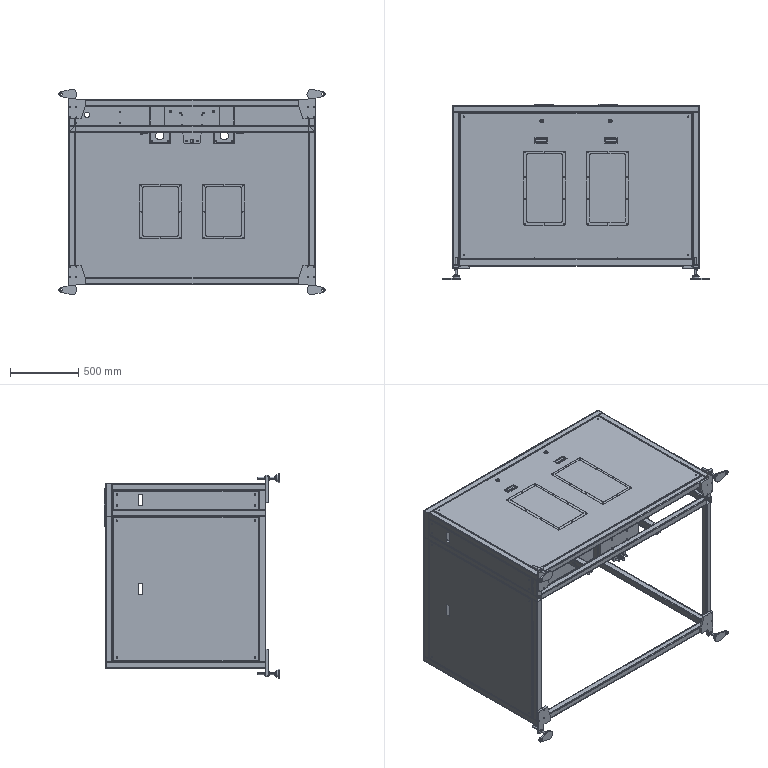Part | SolidWorks | 97 solids | 2489 faces | box 1945 x 1283 x 1500 mm | volume 28861798 mm3 | plane 1128 | cylinder 1105 | cone 164 | spline 92 | commonest cylinder face diameters 6.8 x192 7 x172 25 x119 6 x118 12 x92 5 x80